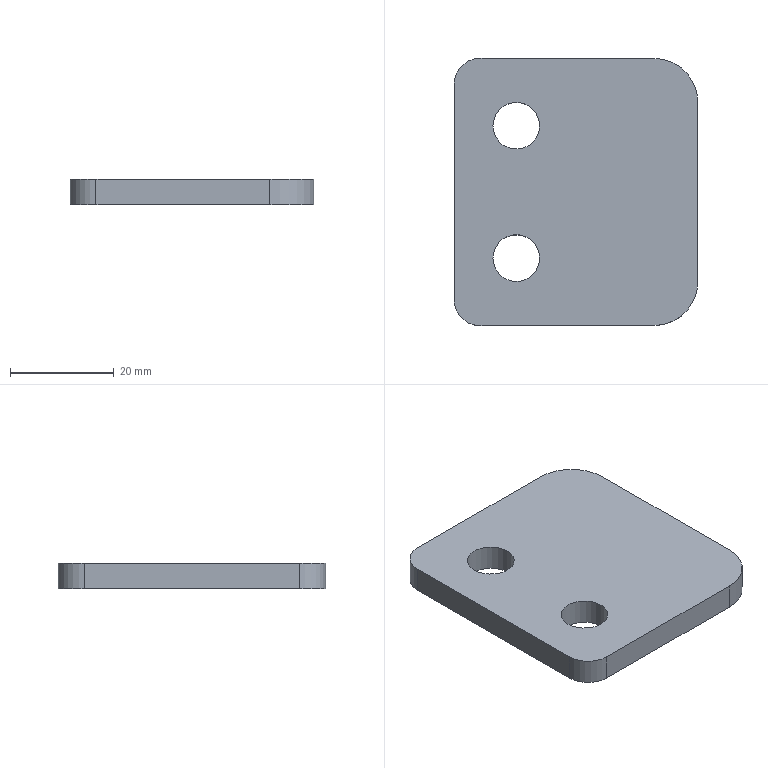Part | STEP file | gslz 2016.10.28-10_id1414_x_t | 1 solid | 12 faces | box 47 x 51.5 x 5 mm | volume 11258 mm3 | cylinder 6 | plane 6 | commonest cylinder face diameters 9 x2 10 x2 17 x2
STEP:
#1=CARTESIAN_POINT('',(0.,0.,0.));
#2=DIRECTION('',(0.,0.,1.));
#3=DIRECTION('',(1.,0.,0.));
#4=AXIS2_PLACEMENT_3D('',#1,#2,#3);
#5=CARTESIAN_POINT('',(-692.25,63.749,15.));
#6=VERTEX_POINT('',#5);
#7=CARTESIAN_POINT('',(-683.75,72.249,15.));
#8=VERTEX_POINT('',#7);
#9=CARTESIAN_POINT('',(-692.25,72.249,15.));
#10=DIRECTION('',(0.,0.,1.));
#11=DIRECTION('',(1.,0.,0.));
#12=AXIS2_PLACEMENT_3D('',#9,#10,#11);
#13=CIRCLE('',#12,8.5);
#14=CARTESIAN_POINT('',(-692.25,72.249,20.));
#15=DIRECTION('',(0.,0.,-1.));
#16=DIRECTION('',(-1.,0.,0.));
#17=AXIS2_PLACEMENT_3D('',#14,#15,#16);
#18=CYLINDRICAL_SURFACE('',#17,8.5);
#19=CARTESIAN_POINT('',(9.425,5.));
#20=DIRECTION('',(-1.,0.));
#21=VECTOR('',#20,1.);
#22=LINE('',#19,#21);
#23=(GEOMETRIC_REPRESENTATION_CONTEXT(2)PARAMETRIC_REPRESENTATION_CONTEXT()REPRESENTATION_CONTEXT('',''));
#24=DEFINITIONAL_REPRESENTATION('',(#22),#23);
#25=PCURVE('',#18,#24);
#26=CARTESIAN_POINT('',(-698.75,87.749,15.));
#27=DIRECTION('',(0.,0.,-1.));
#28=DIRECTION('',(-1.,0.,0.));
#29=AXIS2_PLACEMENT_3D('',#26,#27,#28);
#30=PLANE('',#29);
#31=CARTESIAN_POINT('',(-15.,-15.5));
#32=CARTESIAN_POINT('',(-15.,-0.7776));
#33=CARTESIAN_POINT('',(-2.25,-8.139));
#34=CARTESIAN_POINT('',(10.5,-15.5));
#35=CARTESIAN_POINT('',(-2.25,-22.861));
#36=CARTESIAN_POINT('',(-15.,-30.222));
#37=CARTESIAN_POINT('',(-15.,-15.5));
#38=(BOUNDED_CURVE()B_SPLINE_CURVE(2,(#31,#32,#33,#34,#35,#36,#37),.UNSPECIFIED.,.T.,.F.)B_SPLINE_CURVE_WITH_KNOTS((1,2,2,2,2,1),(-2.094,0.,2.094,4.189,6.283,8.378),.UNSPECIFIED.)CURVE()GEOMETRIC_REPRESENTATION_ITEM()RATIONAL_B_SPLINE_CURVE((1.,0.5,1.,0.5,1.,0.5,1.))REPRESENTATION_ITEM(''));
#39=(GEOMETRIC_REPRESENTATION_CONTEXT(2)PARAMETRIC_REPRESENTATION_CONTEXT()REPRESENTATION_CONTEXT('',''));
#40=DEFINITIONAL_REPRESENTATION('',(#38),#39);
#41=PCURVE('',#30,#40);
#42=SURFACE_CURVE('',#13,(#25,#41),.PCURVE_S1.);
#43=EDGE_CURVE('',#6,#8,#42,.T.);
#44=ORIENTED_EDGE('',*,*,#43,.T.);
#45=CARTESIAN_POINT('',(-683.75,72.249,20.));
#46=VERTEX_POINT('',#45);
#47=CARTESIAN_POINT('',(-683.75,72.249,20.));
#48=DIRECTION('',(0.,0.,-1.));
#49=VECTOR('',#48,1.);
#50=LINE('',#47,#49);
#51=CARTESIAN_POINT('',(3.142,0.));
#52=DIRECTION('',(0.,1.));
#53=VECTOR('',#52,1.);
#54=LINE('',#51,#53);
#55=(GEOMETRIC_REPRESENTATION_CONTEXT(2)PARAMETRIC_REPRESENTATION_CONTEXT()REPRESENTATION_CONTEXT('',''));
#56=DEFINITIONAL_REPRESENTATION('',(#54),#55);
#57=PCURVE('',#18,#56);
#58=CARTESIAN_POINT('',(-683.75,87.749,20.));
#59=DIRECTION('',(-1.,0.,0.));
#60=DIRECTION('',(0.,0.,1.));
#61=AXIS2_PLACEMENT_3D('',#58,#59,#60);
#62=PLANE('',#61);
#63=CARTESIAN_POINT('',(0.,-15.5));
#64=DIRECTION('',(-1.,0.));
#65=VECTOR('',#64,1.);
#66=LINE('',#63,#65);
#67=(GEOMETRIC_REPRESENTATION_CONTEXT(2)PARAMETRIC_REPRESENTATION_CONTEXT()REPRESENTATION_CONTEXT('',''));
#68=DEFINITIONAL_REPRESENTATION('',(#66),#67);
#69=PCURVE('',#62,#68);
#70=SURFACE_CURVE('',#50,(#57,#69),.PCURVE_S1.);
#71=EDGE_CURVE('',#46,#8,#70,.T.);
#72=ORIENTED_EDGE('',*,*,#71,.F.);
#73=CARTESIAN_POINT('',(-692.25,63.749,20.));
#74=VERTEX_POINT('',#73);
#75=CARTESIAN_POINT('',(-692.25,72.249,20.));
#76=DIRECTION('',(0.,0.,1.));
#77=DIRECTION('',(1.,0.,0.));
#78=AXIS2_PLACEMENT_3D('',#75,#76,#77);
#79=CIRCLE('',#78,8.5);
#80=CARTESIAN_POINT('',(9.425,0.));
#81=DIRECTION('',(-1.,0.));
#82=VECTOR('',#81,1.);
#83=LINE('',#80,#82);
#84=(GEOMETRIC_REPRESENTATION_CONTEXT(2)PARAMETRIC_REPRESENTATION_CONTEXT()REPRESENTATION_CONTEXT('',''));
#85=DEFINITIONAL_REPRESENTATION('',(#83),#84);
#86=PCURVE('',#18,#85);
#87=CARTESIAN_POINT('',(-698.75,87.749,20.));
#88=DIRECTION('',(0.,0.,-1.));
#89=DIRECTION('',(-1.,0.,0.));
#90=AXIS2_PLACEMENT_3D('',#87,#88,#89);
#91=PLANE('',#90);
#92=CARTESIAN_POINT('',(-15.,-15.5));
#93=CARTESIAN_POINT('',(-15.,-0.7776));
#94=CARTESIAN_POINT('',(-2.25,-8.139));
#95=CARTESIAN_POINT('',(10.5,-15.5));
#96=CARTESIAN_POINT('',(-2.25,-22.861));
#97=CARTESIAN_POINT('',(-15.,-30.222));
#98=CARTESIAN_POINT('',(-15.,-15.5));
#99=(BOUNDED_CURVE()B_SPLINE_CURVE(2,(#92,#93,#94,#95,#96,#97,#98),.UNSPECIFIED.,.T.,.F.)B_SPLINE_CURVE_WITH_KNOTS((1,2,2,2,2,1),(-2.094,0.,2.094,4.189,6.283,8.378),.UNSPECIFIED.)CURVE()GEOMETRIC_REPRESENTATION_ITEM()RATIONAL_B_SPLINE_CURVE((1.,0.5,1.,0.5,1.,0.5,1.))REPRESENTATION_ITEM(''));
#100=(GEOMETRIC_REPRESENTATION_CONTEXT(2)PARAMETRIC_REPRESENTATION_CONTEXT()REPRESENTATION_CONTEXT('',''));
#101=DEFINITIONAL_REPRESENTATION('',(#99),#100);
#102=PCURVE('',#91,#101);
#103=SURFACE_CURVE('',#79,(#86,#102),.PCURVE_S1.);
#104=EDGE_CURVE('',#74,#46,#103,.T.);
#105=ORIENTED_EDGE('',*,*,#104,.F.);
#106=CARTESIAN_POINT('',(-692.25,63.749,20.));
#107=DIRECTION('',(0.,0.,-1.));
#108=VECTOR('',#107,1.);
#109=LINE('',#106,#108);
#110=CARTESIAN_POINT('',(4.712,0.));
#111=DIRECTION('',(0.,1.));
#112=VECTOR('',#111,1.);
#113=LINE('',#110,#112);
#114=(GEOMETRIC_REPRESENTATION_CONTEXT(2)PARAMETRIC_REPRESENTATION_CONTEXT()REPRESENTATION_CONTEXT('',''));
#115=DEFINITIONAL_REPRESENTATION('',(#113),#114);
#116=PCURVE('',#18,#115);
#117=CARTESIAN_POINT('',(-698.75,63.749,20.));
#118=DIRECTION('',(0.,-1.,0.));
#119=DIRECTION('',(0.,0.,-1.));
#120=AXIS2_PLACEMENT_3D('',#117,#118,#119);
#121=PLANE('',#120);
#122=CARTESIAN_POINT('',(0.,6.5));
#123=DIRECTION('',(1.,0.));
#124=VECTOR('',#123,1.);
#125=LINE('',#122,#124);
#126=(GEOMETRIC_REPRESENTATION_CONTEXT(2)PARAMETRIC_REPRESENTATION_CONTEXT()REPRESENTATION_CONTEXT('',''));
#127=DEFINITIONAL_REPRESENTATION('',(#125),#126);
#128=PCURVE('',#121,#127);
#129=SURFACE_CURVE('',#109,(#116,#128),.PCURVE_S1.);
#130=EDGE_CURVE('',#74,#6,#129,.T.);
#131=ORIENTED_EDGE('',*,*,#130,.T.);
#132=EDGE_LOOP('',(#44,#72,#105,#131));
#133=FACE_BOUND('',#132,.T.);
#134=ADVANCED_FACE('',(#133),#18,.T.);
#135=CARTESIAN_POINT('',(-683.75,106.749,15.));
#136=VERTEX_POINT('',#135);
#137=CARTESIAN_POINT('',(-683.75,87.749,15.));
#138=DIRECTION('',(0.,1.,0.));
#139=VECTOR('',#138,1.);
#140=LINE('',#137,#139);
#141=CARTESIAN_POINT('',(-5.,0.));
#142=DIRECTION('',(0.,1.));
#143=VECTOR('',#142,1.);
#144=LINE('',#141,#143);
#145=(GEOMETRIC_REPRESENTATION_CONTEXT(2)PARAMETRIC_REPRESENTATION_CONTEXT()REPRESENTATION_CONTEXT('',''));
#146=DEFINITIONAL_REPRESENTATION('',(#144),#145);
#147=PCURVE('',#62,#146);
#148=CARTESIAN_POINT('',(-15.,0.));
#149=DIRECTION('',(0.,1.));
#150=VECTOR('',#149,1.);
#151=LINE('',#148,#150);
#152=(GEOMETRIC_REPRESENTATION_CONTEXT(2)PARAMETRIC_REPRESENTATION_CONTEXT()REPRESENTATION_CONTEXT('',''));
#153=DEFINITIONAL_REPRESENTATION('',(#151),#152);
#154=PCURVE('',#30,#153);
#155=SURFACE_CURVE('',#140,(#147,#154),.PCURVE_S1.);
#156=EDGE_CURVE('',#8,#136,#155,.T.);
#157=ORIENTED_EDGE('',*,*,#156,.T.);
#158=CARTESIAN_POINT('',(-683.75,106.749,20.));
#159=VERTEX_POINT('',#158);
#160=CARTESIAN_POINT('',(-683.75,106.749,20.));
#161=DIRECTION('',(0.,0.,-1.));
#162=VECTOR('',#161,1.);
#163=LINE('',#160,#162);
#164=CARTESIAN_POINT('',(0.,19.));
#165=DIRECTION('',(-1.,0.));
#166=VECTOR('',#165,1.);
#167=LINE('',#164,#166);
#168=(GEOMETRIC_REPRESENTATION_CONTEXT(2)PARAMETRIC_REPRESENTATION_CONTEXT()REPRESENTATION_CONTEXT('',''));
#169=DEFINITIONAL_REPRESENTATION('',(#167),#168);
#170=PCURVE('',#62,#169);
#171=CARTESIAN_POINT('',(-692.25,106.749,20.));
#172=DIRECTION('',(0.,0.,-1.));
#173=DIRECTION('',(-1.,0.,0.));
#174=AXIS2_PLACEMENT_3D('',#171,#172,#173);
#175=CYLINDRICAL_SURFACE('',#174,8.5);
#176=CARTESIAN_POINT('',(3.142,0.));
#177=DIRECTION('',(0.,1.));
#178=VECTOR('',#177,1.);
#179=LINE('',#176,#178);
#180=(GEOMETRIC_REPRESENTATION_CONTEXT(2)PARAMETRIC_REPRESENTATION_CONTEXT()REPRESENTATION_CONTEXT('',''));
#181=DEFINITIONAL_REPRESENTATION('',(#179),#180);
#182=PCURVE('',#175,#181);
#183=SURFACE_CURVE('',#163,(#170,#182),.PCURVE_S1.);
#184=EDGE_CURVE('',#159,#136,#183,.T.);
#185=ORIENTED_EDGE('',*,*,#184,.F.);
#186=CARTESIAN_POINT('',(-683.75,87.749,20.));
#187=DIRECTION('',(0.,1.,0.));
#188=VECTOR('',#187,1.);
#189=LINE('',#186,#188);
#190=CARTESIAN_POINT('',(0.,0.));
#191=DIRECTION('',(0.,1.));
#192=VECTOR('',#191,1.);
#193=LINE('',#190,#192);
#194=(GEOMETRIC_REPRESENTATION_CONTEXT(2)PARAMETRIC_REPRESENTATION_CONTEXT()REPRESENTATION_CONTEXT('',''));
#195=DEFINITIONAL_REPRESENTATION('',(#193),#194);
#196=PCURVE('',#62,#195);
#197=CARTESIAN_POINT('',(-15.,0.));
#198=DIRECTION('',(0.,1.));
#199=VECTOR('',#198,1.);
#200=LINE('',#197,#199);
#201=(GEOMETRIC_REPRESENTATION_CONTEXT(2)PARAMETRIC_REPRESENTATION_CONTEXT()REPRESENTATION_CONTEXT('',''));
#202=DEFINITIONAL_REPRESENTATION('',(#200),#201);
#203=PCURVE('',#91,#202);
#204=SURFACE_CURVE('',#189,(#196,#203),.PCURVE_S1.);
#205=EDGE_CURVE('',#46,#159,#204,.T.);
#206=ORIENTED_EDGE('',*,*,#205,.F.);
#207=ORIENTED_EDGE('',*,*,#71,.T.);
#208=EDGE_LOOP('',(#157,#185,#206,#207));
#209=FACE_BOUND('',#208,.T.);
#210=ADVANCED_FACE('',(#209),#62,.F.);
#211=CARTESIAN_POINT('',(-692.25,115.249,15.));
#212=VERTEX_POINT('',#211);
#213=CARTESIAN_POINT('',(-692.25,106.749,15.));
#214=DIRECTION('',(0.,0.,1.));
#215=DIRECTION('',(1.,0.,0.));
#216=AXIS2_PLACEMENT_3D('',#213,#214,#215);
#217=CIRCLE('',#216,8.5);
#218=CARTESIAN_POINT('',(3.142,5.));
#219=DIRECTION('',(-1.,0.));
#220=VECTOR('',#219,1.);
#221=LINE('',#218,#220);
#222=(GEOMETRIC_REPRESENTATION_CONTEXT(2)PARAMETRIC_REPRESENTATION_CONTEXT()REPRESENTATION_CONTEXT('',''));
#223=DEFINITIONAL_REPRESENTATION('',(#221),#222);
#224=PCURVE('',#175,#223);
#225=CARTESIAN_POINT('',(-15.,19.));
#226=CARTESIAN_POINT('',(-15.,33.722));
#227=CARTESIAN_POINT('',(-2.25,26.361));
#228=CARTESIAN_POINT('',(10.5,19.));
#229=CARTESIAN_POINT('',(-2.25,11.639));
#230=CARTESIAN_POINT('',(-15.,4.278));
#231=CARTESIAN_POINT('',(-15.,19.));
#232=(BOUNDED_CURVE()B_SPLINE_CURVE(2,(#225,#226,#227,#228,#229,#230,#231),.UNSPECIFIED.,.T.,.F.)B_SPLINE_CURVE_WITH_KNOTS((1,2,2,2,2,1),(-2.094,0.,2.094,4.189,6.283,8.378),.UNSPECIFIED.)CURVE()GEOMETRIC_REPRESENTATION_ITEM()RATIONAL_B_SPLINE_CURVE((1.,0.5,1.,0.5,1.,0.5,1.))REPRESENTATION_ITEM(''));
#233=(GEOMETRIC_REPRESENTATION_CONTEXT(2)PARAMETRIC_REPRESENTATION_CONTEXT()REPRESENTATION_CONTEXT('',''));
#234=DEFINITIONAL_REPRESENTATION('',(#232),#233);
#235=PCURVE('',#30,#234);
#236=SURFACE_CURVE('',#217,(#224,#235),.PCURVE_S1.);
#237=EDGE_CURVE('',#136,#212,#236,.T.);
#238=ORIENTED_EDGE('',*,*,#237,.T.);
#239=CARTESIAN_POINT('',(-692.25,115.249,20.));
#240=VERTEX_POINT('',#239);
#241=CARTESIAN_POINT('',(-692.25,115.249,20.));
#242=DIRECTION('',(0.,0.,-1.));
#243=VECTOR('',#242,1.);
#244=LINE('',#241,#243);
#245=CARTESIAN_POINT('',(1.571,0.));
#246=DIRECTION('',(0.,1.));
#247=VECTOR('',#246,1.);
#248=LINE('',#245,#247);
#249=(GEOMETRIC_REPRESENTATION_CONTEXT(2)PARAMETRIC_REPRESENTATION_CONTEXT()REPRESENTATION_CONTEXT('',''));
#250=DEFINITIONAL_REPRESENTATION('',(#248),#249);
#251=PCURVE('',#175,#250);
#252=CARTESIAN_POINT('',(-698.75,115.249,20.));
#253=DIRECTION('',(0.,1.,0.));
#254=DIRECTION('',(0.,0.,1.));
#255=AXIS2_PLACEMENT_3D('',#252,#253,#254);
#256=PLANE('',#255);
#257=CARTESIAN_POINT('',(0.,6.5));
#258=DIRECTION('',(-1.,0.));
#259=VECTOR('',#258,1.);
#260=LINE('',#257,#259);
#261=(GEOMETRIC_REPRESENTATION_CONTEXT(2)PARAMETRIC_REPRESENTATION_CONTEXT()REPRESENTATION_CONTEXT('',''));
#262=DEFINITIONAL_REPRESENTATION('',(#260),#261);
#263=PCURVE('',#256,#262);
#264=SURFACE_CURVE('',#244,(#251,#263),.PCURVE_S1.);
#265=EDGE_CURVE('',#240,#212,#264,.T.);
#266=ORIENTED_EDGE('',*,*,#265,.F.);
#267=CARTESIAN_POINT('',(-692.25,106.749,20.));
#268=DIRECTION('',(0.,0.,1.));
#269=DIRECTION('',(1.,0.,0.));
#270=AXIS2_PLACEMENT_3D('',#267,#268,#269);
#271=CIRCLE('',#270,8.5);
#272=CARTESIAN_POINT('',(3.142,0.));
#273=DIRECTION('',(-1.,0.));
#274=VECTOR('',#273,1.);
#275=LINE('',#272,#274);
#276=(GEOMETRIC_REPRESENTATION_CONTEXT(2)PARAMETRIC_REPRESENTATION_CONTEXT()REPRESENTATION_CONTEXT('',''));
#277=DEFINITIONAL_REPRESENTATION('',(#275),#276);
#278=PCURVE('',#175,#277);
#279=CARTESIAN_POINT('',(-15.,19.));
#280=CARTESIAN_POINT('',(-15.,33.722));
#281=CARTESIAN_POINT('',(-2.25,26.361));
#282=CARTESIAN_POINT('',(10.5,19.));
#283=CARTESIAN_POINT('',(-2.25,11.639));
#284=CARTESIAN_POINT('',(-15.,4.278));
#285=CARTESIAN_POINT('',(-15.,19.));
#286=(BOUNDED_CURVE()B_SPLINE_CURVE(2,(#279,#280,#281,#282,#283,#284,#285),.UNSPECIFIED.,.T.,.F.)B_SPLINE_CURVE_WITH_KNOTS((1,2,2,2,2,1),(-2.094,0.,2.094,4.189,6.283,8.378),.UNSPECIFIED.)CURVE()GEOMETRIC_REPRESENTATION_ITEM()RATIONAL_B_SPLINE_CURVE((1.,0.5,1.,0.5,1.,0.5,1.))REPRESENTATION_ITEM(''));
#287=(GEOMETRIC_REPRESENTATION_CONTEXT(2)PARAMETRIC_REPRESENTATION_CONTEXT()REPRESENTATION_CONTEXT('',''));
#288=DEFINITIONAL_REPRESENTATION('',(#286),#287);
#289=PCURVE('',#91,#288);
#290=SURFACE_CURVE('',#271,(#278,#289),.PCURVE_S1.);
#291=EDGE_CURVE('',#159,#240,#290,.T.);
#292=ORIENTED_EDGE('',*,*,#291,.F.);
#293=ORIENTED_EDGE('',*,*,#184,.T.);
#294=EDGE_LOOP('',(#238,#266,#292,#293));
#295=FACE_BOUND('',#294,.T.);
#296=ADVANCED_FACE('',(#295),#175,.T.);
#297=CARTESIAN_POINT('',(-725.75,115.249,15.));
#298=VERTEX_POINT('',#297);
#299=CARTESIAN_POINT('',(-698.75,115.249,15.));
#300=DIRECTION('',(1.,0.,0.));
#301=VECTOR('',#300,1.);
#302=LINE('',#299,#301);
#303=CARTESIAN_POINT('',(-5.,0.));
#304=DIRECTION('',(0.,1.));
#305=VECTOR('',#304,1.);
#306=LINE('',#303,#305);
#307=(GEOMETRIC_REPRESENTATION_CONTEXT(2)PARAMETRIC_REPRESENTATION_CONTEXT()REPRESENTATION_CONTEXT('',''));
#308=DEFINITIONAL_REPRESENTATION('',(#306),#307);
#309=PCURVE('',#256,#308);
#310=CARTESIAN_POINT('',(0.,27.5));
#311=DIRECTION('',(-1.,0.));
#312=VECTOR('',#311,1.);
#313=LINE('',#310,#312);
#314=(GEOMETRIC_REPRESENTATION_CONTEXT(2)PARAMETRIC_REPRESENTATION_CONTEXT()REPRESENTATION_CONTEXT('',''));
#315=DEFINITIONAL_REPRESENTATION('',(#313),#314);
#316=PCURVE('',#30,#315);
#317=SURFACE_CURVE('',#302,(#309,#316),.PCURVE_S1.);
#318=EDGE_CURVE('',#298,#212,#317,.T.);
#319=ORIENTED_EDGE('',*,*,#318,.F.);
#320=CARTESIAN_POINT('',(-725.75,115.249,20.));
#321=VERTEX_POINT('',#320);
#322=CARTESIAN_POINT('',(-725.75,115.249,20.));
#323=DIRECTION('',(0.,0.,-1.));
#324=VECTOR('',#323,1.);
#325=LINE('',#322,#324);
#326=CARTESIAN_POINT('',(0.,-27.));
#327=DIRECTION('',(-1.,0.));
#328=VECTOR('',#327,1.);
#329=LINE('',#326,#328);
#330=(GEOMETRIC_REPRESENTATION_CONTEXT(2)PARAMETRIC_REPRESENTATION_CONTEXT()REPRESENTATION_CONTEXT('',''));
#331=DEFINITIONAL_REPRESENTATION('',(#329),#330);
#332=PCURVE('',#256,#331);
#333=CARTESIAN_POINT('',(-725.75,110.249,20.));
#334=DIRECTION('',(0.,0.,-1.));
#335=DIRECTION('',(-1.,0.,0.));
#336=AXIS2_PLACEMENT_3D('',#333,#334,#335);
#337=CYLINDRICAL_SURFACE('',#336,5.);
#338=CARTESIAN_POINT('',(1.571,0.));
#339=DIRECTION('',(0.,1.));
#340=VECTOR('',#339,1.);
#341=LINE('',#338,#340);
#342=(GEOMETRIC_REPRESENTATION_CONTEXT(2)PARAMETRIC_REPRESENTATION_CONTEXT()REPRESENTATION_CONTEXT('',''));
#343=DEFINITIONAL_REPRESENTATION('',(#341),#342);
#344=PCURVE('',#337,#343);
#345=SURFACE_CURVE('',#325,(#332,#344),.PCURVE_S1.);
#346=EDGE_CURVE('',#321,#298,#345,.T.);
#347=ORIENTED_EDGE('',*,*,#346,.F.);
#348=CARTESIAN_POINT('',(-698.75,115.249,20.));
#349=DIRECTION('',(1.,0.,0.));
#350=VECTOR('',#349,1.);
#351=LINE('',#348,#350);
#352=CARTESIAN_POINT('',(0.,0.));
#353=DIRECTION('',(0.,1.));
#354=VECTOR('',#353,1.);
#355=LINE('',#352,#354);
#356=(GEOMETRIC_REPRESENTATION_CONTEXT(2)PARAMETRIC_REPRESENTATION_CONTEXT()REPRESENTATION_CONTEXT('',''));
#357=DEFINITIONAL_REPRESENTATION('',(#355),#356);
#358=PCURVE('',#256,#357);
#359=CARTESIAN_POINT('',(0.,27.5));
#360=DIRECTION('',(-1.,0.));
#361=VECTOR('',#360,1.);
#362=LINE('',#359,#361);
#363=(GEOMETRIC_REPRESENTATION_CONTEXT(2)PARAMETRIC_REPRESENTATION_CONTEXT()REPRESENTATION_CONTEXT('',''));
#364=DEFINITIONAL_REPRESENTATION('',(#362),#363);
#365=PCURVE('',#91,#364);
#366=SURFACE_CURVE('',#351,(#358,#365),.PCURVE_S1.);
#367=EDGE_CURVE('',#321,#240,#366,.T.);
#368=ORIENTED_EDGE('',*,*,#367,.T.);
#369=ORIENTED_EDGE('',*,*,#265,.T.);
#370=EDGE_LOOP('',(#319,#347,#368,#369));
#371=FACE_BOUND('',#370,.T.);
#372=ADVANCED_FACE('',(#371),#256,.T.);
#373=CARTESIAN_POINT('',(-730.75,110.249,15.));
#374=VERTEX_POINT('',#373);
#375=CARTESIAN_POINT('',(-725.75,110.249,15.));
#376=DIRECTION('',(0.,0.,1.));
#377=DIRECTION('',(1.,0.,0.));
#378=AXIS2_PLACEMENT_3D('',#375,#376,#377);
#379=CIRCLE('',#378,5.);
#380=CARTESIAN_POINT('',(3.142,5.));
#381=DIRECTION('',(-1.,0.));
#382=VECTOR('',#381,1.);
#383=LINE('',#380,#382);
#384=(GEOMETRIC_REPRESENTATION_CONTEXT(2)PARAMETRIC_REPRESENTATION_CONTEXT()REPRESENTATION_CONTEXT('',''));
#385=DEFINITIONAL_REPRESENTATION('',(#383),#384);
#386=PCURVE('',#337,#385);
#387=CARTESIAN_POINT('',(22.,22.5));
#388=CARTESIAN_POINT('',(22.,31.16));
#389=CARTESIAN_POINT('',(29.5,26.83));
#390=CARTESIAN_POINT('',(37.,22.5));
#391=CARTESIAN_POINT('',(29.5,18.17));
#392=CARTESIAN_POINT('',(22.,13.84));
#393=CARTESIAN_POINT('',(22.,22.5));
#394=(BOUNDED_CURVE()B_SPLINE_CURVE(2,(#387,#388,#389,#390,#391,#392,#393),.UNSPECIFIED.,.T.,.F.)B_SPLINE_CURVE_WITH_KNOTS((1,2,2,2,2,1),(-2.094,0.,2.094,4.189,6.283,8.378),.UNSPECIFIED.)CURVE()GEOMETRIC_REPRESENTATION_ITEM()RATIONAL_B_SPLINE_CURVE((1.,0.5,1.,0.5,1.,0.5,1.))REPRESENTATION_ITEM(''));
#395=(GEOMETRIC_REPRESENTATION_CONTEXT(2)PARAMETRIC_REPRESENTATION_CONTEXT()REPRESENTATION_CONTEXT('',''));
#396=DEFINITIONAL_REPRESENTATION('',(#394),#395);
#397=PCURVE('',#30,#396);
#398=SURFACE_CURVE('',#379,(#386,#397),.PCURVE_S1.);
#399=EDGE_CURVE('',#298,#374,#398,.T.);
#400=ORIENTED_EDGE('',*,*,#399,.T.);
#401=CARTESIAN_POINT('',(-730.75,110.249,20.));
#402=VERTEX_POINT('',#401);
#403=CARTESIAN_POINT('',(-730.75,110.249,20.));
#404=DIRECTION('',(0.,0.,-1.));
#405=VECTOR('',#404,1.);
#406=LINE('',#403,#405);
#407=CARTESIAN_POINT('',(0.,0.));
#408=DIRECTION('',(0.,1.));
#409=VECTOR('',#408,1.);
#410=LINE('',#407,#409);
#411=(GEOMETRIC_REPRESENTATION_CONTEXT(2)PARAMETRIC_REPRESENTATION_CONTEXT()REPRESENTATION_CONTEXT('',''));
#412=DEFINITIONAL_REPRESENTATION('',(#410),#411);
#413=PCURVE('',#337,#412);
#414=CARTESIAN_POINT('',(-730.75,87.749,20.));
#415=DIRECTION('',(-1.,0.,0.));
#416=DIRECTION('',(0.,0.,1.));
#417=AXIS2_PLACEMENT_3D('',#414,#415,#416);
#418=PLANE('',#417);
#419=CARTESIAN_POINT('',(0.,22.5));
#420=DIRECTION('',(-1.,0.));
#421=VECTOR('',#420,1.);
#422=LINE('',#419,#421);
#423=(GEOMETRIC_REPRESENTATION_CONTEXT(2)PARAMETRIC_REPRESENTATION_CONTEXT()REPRESENTATION_CONTEXT('',''));
#424=DEFINITIONAL_REPRESENTATION('',(#422),#423);
#425=PCURVE('',#418,#424);
#426=SURFACE_CURVE('',#406,(#413,#425),.PCURVE_S1.);
#427=EDGE_CURVE('',#402,#374,#426,.T.);
#428=ORIENTED_EDGE('',*,*,#427,.F.);
#429=CARTESIAN_POINT('',(-725.75,110.249,20.));
#430=DIRECTION('',(0.,0.,1.));
#431=DIRECTION('',(1.,0.,0.));
#432=AXIS2_PLACEMENT_3D('',#429,#430,#431);
#433=CIRCLE('',#432,5.);
#434=CARTESIAN_POINT('',(3.142,0.));
#435=DIRECTION('',(-1.,0.));
#436=VECTOR('',#435,1.);
#437=LINE('',#434,#436);
#438=(GEOMETRIC_REPRESENTATION_CONTEXT(2)PARAMETRIC_REPRESENTATION_CONTEXT()REPRESENTATION_CONTEXT('',''));
#439=DEFINITIONAL_REPRESENTATION('',(#437),#438);
#440=PCURVE('',#337,#439);
#441=CARTESIAN_POINT('',(22.,22.5));
#442=CARTESIAN_POINT('',(22.,31.16));
#443=CARTESIAN_POINT('',(29.5,26.83));
#444=CARTESIAN_POINT('',(37.,22.5));
#445=CARTESIAN_POINT('',(29.5,18.17));
#446=CARTESIAN_POINT('',(22.,13.84));
#447=CARTESIAN_POINT('',(22.,22.5));
#448=(BOUNDED_CURVE()B_SPLINE_CURVE(2,(#441,#442,#443,#444,#445,#446,#447),.UNSPECIFIED.,.T.,.F.)B_SPLINE_CURVE_WITH_KNOTS((1,2,2,2,2,1),(-2.094,0.,2.094,4.189,6.283,8.378),.UNSPECIFIED.)CURVE()GEOMETRIC_REPRESENTATION_ITEM()RATIONAL_B_SPLINE_CURVE((1.,0.5,1.,0.5,1.,0.5,1.))REPRESENTATION_ITEM(''));
#449=(GEOMETRIC_REPRESENTATION_CONTEXT(2)PARAMETRIC_REPRESENTATION_CONTEXT()REPRESENTATION_CONTEXT('',''));
#450=DEFINITIONAL_REPRESENTATION('',(#448),#449);
#451=PCURVE('',#91,#450);
#452=SURFACE_CURVE('',#433,(#440,#451),.PCURVE_S1.);
#453=EDGE_CURVE('',#321,#402,#452,.T.);
#454=ORIENTED_EDGE('',*,*,#453,.F.);
#455=ORIENTED_EDGE('',*,*,#346,.T.);
#456=EDGE_LOOP('',(#400,#428,#454,#455));
#457=FACE_BOUND('',#456,.T.);
#458=ADVANCED_FACE('',(#457),#337,.T.);
#459=CARTESIAN_POINT('',(-730.75,68.749,15.));
#460=VERTEX_POINT('',#459);
#461=CARTESIAN_POINT('',(-730.75,87.749,15.));
#462=DIRECTION('',(0.,1.,0.));
#463=VECTOR('',#462,1.);
#464=LINE('',#461,#463);
#465=CARTESIAN_POINT('',(-5.,0.));
#466=DIRECTION('',(0.,1.));
#467=VECTOR('',#466,1.);
#468=LINE('',#465,#467);
#469=(GEOMETRIC_REPRESENTATION_CONTEXT(2)PARAMETRIC_REPRESENTATION_CONTEXT()REPRESENTATION_CONTEXT('',''));
#470=DEFINITIONAL_REPRESENTATION('',(#468),#469);
#471=PCURVE('',#418,#470);
#472=CARTESIAN_POINT('',(32.,0.));
#473=DIRECTION('',(0.,1.));
#474=VECTOR('',#473,1.);
#475=LINE('',#472,#474);
#476=(GEOMETRIC_REPRESENTATION_CONTEXT(2)PARAMETRIC_REPRESENTATION_CONTEXT()REPRESENTATION_CONTEXT('',''));
#477=DEFINITIONAL_REPRESENTATION('',(#475),#476);
#478=PCURVE('',#30,#477);
#479=SURFACE_CURVE('',#464,(#471,#478),.PCURVE_S1.);
#480=EDGE_CURVE('',#460,#374,#479,.T.);
#481=ORIENTED_EDGE('',*,*,#480,.F.);
#482=CARTESIAN_POINT('',(-730.75,68.749,20.));
#483=VERTEX_POINT('',#482);
#484=CARTESIAN_POINT('',(-730.75,68.749,20.));
#485=DIRECTION('',(0.,0.,-1.));
#486=VECTOR('',#485,1.);
#487=LINE('',#484,#486);
#488=CARTESIAN_POINT('',(0.,-19.));
#489=DIRECTION('',(-1.,0.));
#490=VECTOR('',#489,1.);
#491=LINE('',#488,#490);
#492=(GEOMETRIC_REPRESENTATION_CONTEXT(2)PARAMETRIC_REPRESENTATION_CONTEXT()REPRESENTATION_CONTEXT('',''));
#493=DEFINITIONAL_REPRESENTATION('',(#491),#492);
#494=PCURVE('',#418,#493);
#495=CARTESIAN_POINT('',(-725.75,68.749,20.));
#496=DIRECTION('',(0.,0.,-1.));
#497=DIRECTION('',(-1.,0.,0.));
#498=AXIS2_PLACEMENT_3D('',#495,#496,#497);
#499=CYLINDRICAL_SURFACE('',#498,5.);
#500=CARTESIAN_POINT('',(6.283,0.));
#501=DIRECTION('',(0.,1.));
#502=VECTOR('',#501,1.);
#503=LINE('',#500,#502);
#504=(GEOMETRIC_REPRESENTATION_CONTEXT(2)PARAMETRIC_REPRESENTATION_CONTEXT()REPRESENTATION_CONTEXT('',''));
#505=DEFINITIONAL_REPRESENTATION('',(#503),#504);
#506=PCURVE('',#499,#505);
#507=SURFACE_CURVE('',#487,(#494,#506),.PCURVE_S1.);
#508=EDGE_CURVE('',#483,#460,#507,.T.);
#509=ORIENTED_EDGE('',*,*,#508,.F.);
#510=CARTESIAN_POINT('',(-730.75,87.749,20.));
#511=DIRECTION('',(0.,1.,0.));
#512=VECTOR('',#511,1.);
#513=LINE('',#510,#512);
#514=CARTESIAN_POINT('',(0.,0.));
#515=DIRECTION('',(0.,1.));
#516=VECTOR('',#515,1.);
#517=LINE('',#514,#516);
#518=(GEOMETRIC_REPRESENTATION_CONTEXT(2)PARAMETRIC_REPRESENTATION_CONTEXT()REPRESENTATION_CONTEXT('',''));
#519=DEFINITIONAL_REPRESENTATION('',(#517),#518);
#520=PCURVE('',#418,#519);
#521=CARTESIAN_POINT('',(32.,0.));
#522=DIRECTION('',(0.,1.));
#523=VECTOR('',#522,1.);
#524=LINE('',#521,#523);
#525=(GEOMETRIC_REPRESENTATION_CONTEXT(2)PARAMETRIC_REPRESENTATION_CONTEXT()REPRESENTATION_CONTEXT('',''));
#526=DEFINITIONAL_REPRESENTATION('',(#524),#525);
#527=PCURVE('',#91,#526);
#528=SURFACE_CURVE('',#513,(#520,#527),.PCURVE_S1.);
#529=EDGE_CURVE('',#483,#402,#528,.T.);
#530=ORIENTED_EDGE('',*,*,#529,.T.);
#531=ORIENTED_EDGE('',*,*,#427,.T.);
#532=EDGE_LOOP('',(#481,#509,#530,#531));
#533=FACE_BOUND('',#532,.T.);
#534=ADVANCED_FACE('',(#533),#418,.T.);
#535=CARTESIAN_POINT('',(-725.75,63.749,15.));
#536=VERTEX_POINT('',#535);
#537=CARTESIAN_POINT('',(-725.75,68.749,15.));
#538=DIRECTION('',(0.,0.,1.));
#539=DIRECTION('',(1.,0.,0.));
#540=AXIS2_PLACEMENT_3D('',#537,#538,#539);
#541=CIRCLE('',#540,5.);
#542=CARTESIAN_POINT('',(9.425,5.));
#543=DIRECTION('',(-1.,0.));
#544=VECTOR('',#543,1.);
#545=LINE('',#542,#544);
#546=(GEOMETRIC_REPRESENTATION_CONTEXT(2)PARAMETRIC_REPRESENTATION_CONTEXT()REPRESENTATION_CONTEXT('',''));
#547=DEFINITIONAL_REPRESENTATION('',(#545),#546);
#548=PCURVE('',#499,#547);
#549=CARTESIAN_POINT('',(22.,-19.));
#550=CARTESIAN_POINT('',(22.,-10.34));
#551=CARTESIAN_POINT('',(29.5,-14.67));
#552=CARTESIAN_POINT('',(37.,-19.));
#553=CARTESIAN_POINT('',(29.5,-23.33));
#554=CARTESIAN_POINT('',(22.,-27.66));
#555=CARTESIAN_POINT('',(22.,-19.));
#556=(BOUNDED_CURVE()B_SPLINE_CURVE(2,(#549,#550,#551,#552,#553,#554,#555),.UNSPECIFIED.,.T.,.F.)B_SPLINE_CURVE_WITH_KNOTS((1,2,2,2,2,1),(-2.094,0.,2.094,4.189,6.283,8.378),.UNSPECIFIED.)CURVE()GEOMETRIC_REPRESENTATION_ITEM()RATIONAL_B_SPLINE_CURVE((1.,0.5,1.,0.5,1.,0.5,1.))REPRESENTATION_ITEM(''));
#557=(GEOMETRIC_REPRESENTATION_CONTEXT(2)PARAMETRIC_REPRESENTATION_CONTEXT()REPRESENTATION_CONTEXT('',''));
#558=DEFINITIONAL_REPRESENTATION('',(#556),#557);
#559=PCURVE('',#30,#558);
#560=SURFACE_CURVE('',#541,(#548,#559),.PCURVE_S1.);
#561=EDGE_CURVE('',#460,#536,#560,.T.);
#562=ORIENTED_EDGE('',*,*,#561,.T.);
#563=CARTESIAN_POINT('',(-725.75,63.749,20.));
#564=VERTEX_POINT('',#563);
#565=CARTESIAN_POINT('',(-725.75,63.749,20.));
#566=DIRECTION('',(0.,0.,-1.));
#567=VECTOR('',#566,1.);
#568=LINE('',#565,#567);
#569=CARTESIAN_POINT('',(4.712,0.));
#570=DIRECTION('',(0.,1.));
#571=VECTOR('',#570,1.);
#572=LINE('',#569,#571);
#573=(GEOMETRIC_REPRESENTATION_CONTEXT(2)PARAMETRIC_REPRESENTATION_CONTEXT()REPRESENTATION_CONTEXT('',''));
#574=DEFINITIONAL_REPRESENTATION('',(#572),#573);
#575=PCURVE('',#499,#574);
#576=CARTESIAN_POINT('',(0.,-27.));
#577=DIRECTION('',(1.,0.));
#578=VECTOR('',#577,1.);
#579=LINE('',#576,#578);
#580=(GEOMETRIC_REPRESENTATION_CONTEXT(2)PARAMETRIC_REPRESENTATION_CONTEXT()REPRESENTATION_CONTEXT('',''));
#581=DEFINITIONAL_REPRESENTATION('',(#579),#580);
#582=PCURVE('',#121,#581);
#583=SURFACE_CURVE('',#568,(#575,#582),.PCURVE_S1.);
#584=EDGE_CURVE('',#564,#536,#583,.T.);
#585=ORIENTED_EDGE('',*,*,#584,.F.);
#586=CARTESIAN_POINT('',(-725.75,68.749,20.));
#587=DIRECTION('',(0.,0.,1.));
#588=DIRECTION('',(1.,0.,0.));
#589=AXIS2_PLACEMENT_3D('',#586,#587,#588);
#590=CIRCLE('',#589,5.);
#591=CARTESIAN_POINT('',(9.425,0.));
#592=DIRECTION('',(-1.,0.));
#593=VECTOR('',#592,1.);
#594=LINE('',#591,#593);
#595=(GEOMETRIC_REPRESENTATION_CONTEXT(2)PARAMETRIC_REPRESENTATION_CONTEXT()REPRESENTATION_CONTEXT('',''));
#596=DEFINITIONAL_REPRESENTATION('',(#594),#595);
#597=PCURVE('',#499,#596);
#598=CARTESIAN_POINT('',(22.,-19.));
#599=CARTESIAN_POINT('',(22.,-10.34));
#600=CARTESIAN_POINT('',(29.5,-14.67));
#601=CARTESIAN_POINT('',(37.,-19.));
#602=CARTESIAN_POINT('',(29.5,-23.33));
#603=CARTESIAN_POINT('',(22.,-27.66));
#604=CARTESIAN_POINT('',(22.,-19.));
#605=(BOUNDED_CURVE()B_SPLINE_CURVE(2,(#598,#599,#600,#601,#602,#603,#604),.UNSPECIFIED.,.T.,.F.)B_SPLINE_CURVE_WITH_KNOTS((1,2,2,2,2,1),(-2.094,0.,2.094,4.189,6.283,8.378),.UNSPECIFIED.)CURVE()GEOMETRIC_REPRESENTATION_ITEM()RATIONAL_B_SPLINE_CURVE((1.,0.5,1.,0.5,1.,0.5,1.))REPRESENTATION_ITEM(''));
#606=(GEOMETRIC_REPRESENTATION_CONTEXT(2)PARAMETRIC_REPRESENTATION_CONTEXT()REPRESENTATION_CONTEXT('',''));
#607=DEFINITIONAL_REPRESENTATION('',(#605),#606);
#608=PCURVE('',#91,#607);
#609=SURFACE_CURVE('',#590,(#597,#608),.PCURVE_S1.);
#610=EDGE_CURVE('',#483,#564,#609,.T.);
#611=ORIENTED_EDGE('',*,*,#610,.F.);
#612=ORIENTED_EDGE('',*,*,#508,.T.);
#613=EDGE_LOOP('',(#562,#585,#611,#612));
#614=FACE_BOUND('',#613,.T.);
#615=ADVANCED_FACE('',(#614),#499,.T.);
#616=CARTESIAN_POINT('',(-723.25,102.249,20.));
#617=VERTEX_POINT('',#616);
#618=CARTESIAN_POINT('',(-718.75,102.249,20.));
#619=DIRECTION('',(0.,0.,-1.));
#620=DIRECTION('',(-1.,0.,0.));
#621=AXIS2_PLACEMENT_3D('',#618,#619,#620);
#622=CIRCLE('',#621,4.5);
#623=CARTESIAN_POINT('',(-718.75,102.249,20.));
#624=DIRECTION('',(0.,0.,-1.));
#625=DIRECTION('',(-1.,0.,0.));
#626=AXIS2_PLACEMENT_3D('',#623,#624,#625);
#627=CYLINDRICAL_SURFACE('',#626,4.5);
#628=CARTESIAN_POINT('',(0.,0.));
#629=DIRECTION('',(1.,0.));
#630=VECTOR('',#629,1.);
#631=LINE('',#628,#630);
#632=(GEOMETRIC_REPRESENTATION_CONTEXT(2)PARAMETRIC_REPRESENTATION_CONTEXT()REPRESENTATION_CONTEXT('',''));
#633=DEFINITIONAL_REPRESENTATION('',(#631),#632);
#634=PCURVE('',#627,#633);
#635=CARTESIAN_POINT('',(20.,14.5));
#636=DIRECTION('',(1.,0.));
#637=AXIS2_PLACEMENT_2D('',#635,#636);
#638=CIRCLE('',#637,4.5);
#639=(GEOMETRIC_REPRESENTATION_CONTEXT(2)PARAMETRIC_REPRESENTATION_CONTEXT()REPRESENTATION_CONTEXT('',''));
#640=DEFINITIONAL_REPRESENTATION('',(#638),#639);
#641=PCURVE('',#91,#640);
#642=SURFACE_CURVE('',#622,(#634,#641),.PCURVE_S1.);
#643=EDGE_CURVE('',#617,#617,#642,.T.);
#644=ORIENTED_EDGE('',*,*,#643,.T.);
#645=CARTESIAN_POINT('',(-723.25,102.249,15.));
#646=VERTEX_POINT('',#645);
#647=CARTESIAN_POINT('',(-723.25,102.249,20.));
#648=CARTESIAN_POINT('',(-723.25,102.249,15.));
#649=B_SPLINE_CURVE_WITH_KNOTS('',1,(#647,#648),.UNSPECIFIED.,.F.,.F.,(2,2),(0.,5.),.PIECEWISE_BEZIER_KNOTS.);
#650=CARTESIAN_POINT('',(6.283,0.));
#651=DIRECTION('',(0.,1.));
#652=VECTOR('',#651,1.);
#653=LINE('',#650,#652);
#654=(GEOMETRIC_REPRESENTATION_CONTEXT(2)PARAMETRIC_REPRESENTATION_CONTEXT()REPRESENTATION_CONTEXT('',''));
#655=DEFINITIONAL_REPRESENTATION('',(#653),#654);
#656=PCURVE('',#627,#655);
#657=CARTESIAN_POINT('',(0.,0.));
#658=DIRECTION('',(0.,1.));
#659=VECTOR('',#658,1.);
#660=LINE('',#657,#659);
#661=(GEOMETRIC_REPRESENTATION_CONTEXT(2)PARAMETRIC_REPRESENTATION_CONTEXT()REPRESENTATION_CONTEXT('',''));
#662=DEFINITIONAL_REPRESENTATION('',(#660),#661);
#663=PCURVE('',#627,#662);
#664=SEAM_CURVE('',#649,(#656,#663),.PCURVE_S1.);
#665=EDGE_CURVE('',#617,#646,#664,.T.);
#666=ORIENTED_EDGE('',*,*,#665,.T.);
#667=CARTESIAN_POINT('',(-718.75,102.249,15.));
#668=DIRECTION('',(0.,0.,-1.));
#669=DIRECTION('',(-1.,0.,0.));
#670=AXIS2_PLACEMENT_3D('',#667,#668,#669);
#671=CIRCLE('',#670,4.5);
#672=CARTESIAN_POINT('',(0.,5.));
#673=DIRECTION('',(1.,0.));
#674=VECTOR('',#673,1.);
#675=LINE('',#672,#674);
#676=(GEOMETRIC_REPRESENTATION_CONTEXT(2)PARAMETRIC_REPRESENTATION_CONTEXT()REPRESENTATION_CONTEXT('',''));
#677=DEFINITIONAL_REPRESENTATION('',(#675),#676);
#678=PCURVE('',#627,#677);
#679=CARTESIAN_POINT('',(20.,14.5));
#680=DIRECTION('',(1.,0.));
#681=AXIS2_PLACEMENT_2D('',#679,#680);
#682=CIRCLE('',#681,4.5);
#683=(GEOMETRIC_REPRESENTATION_CONTEXT(2)PARAMETRIC_REPRESENTATION_CONTEXT()REPRESENTATION_CONTEXT('',''));
#684=DEFINITIONAL_REPRESENTATION('',(#682),#683);
#685=PCURVE('',#30,#684);
#686=SURFACE_CURVE('',#671,(#678,#685),.PCURVE_S1.);
#687=EDGE_CURVE('',#646,#646,#686,.T.);
#688=ORIENTED_EDGE('',*,*,#687,.F.);
#689=ORIENTED_EDGE('',*,*,#665,.F.);
#690=EDGE_LOOP('',(#644,#666,#688,#689));
#691=FACE_BOUND('',#690,.F.);
#692=ADVANCED_FACE('',(#691),#627,.F.);
#693=CARTESIAN_POINT('',(-723.25,76.749,20.));
#694=VERTEX_POINT('',#693);
#695=CARTESIAN_POINT('',(-718.75,76.749,20.));
#696=DIRECTION('',(0.,0.,-1.));
#697=DIRECTION('',(-1.,0.,0.));
#698=AXIS2_PLACEMENT_3D('',#695,#696,#697);
#699=CIRCLE('',#698,4.5);
#700=CARTESIAN_POINT('',(-718.75,76.749,20.));
#701=DIRECTION('',(0.,0.,-1.));
#702=DIRECTION('',(-1.,0.,0.));
#703=AXIS2_PLACEMENT_3D('',#700,#701,#702);
#704=CYLINDRICAL_SURFACE('',#703,4.5);
#705=CARTESIAN_POINT('',(0.,0.));
#706=DIRECTION('',(1.,0.));
#707=VECTOR('',#706,1.);
#708=LINE('',#705,#707);
#709=(GEOMETRIC_REPRESENTATION_CONTEXT(2)PARAMETRIC_REPRESENTATION_CONTEXT()REPRESENTATION_CONTEXT('',''));
#710=DEFINITIONAL_REPRESENTATION('',(#708),#709);
#711=PCURVE('',#704,#710);
#712=CARTESIAN_POINT('',(20.,-11.));
#713=DIRECTION('',(1.,0.));
#714=AXIS2_PLACEMENT_2D('',#712,#713);
#715=CIRCLE('',#714,4.5);
#716=(GEOMETRIC_REPRESENTATION_CONTEXT(2)PARAMETRIC_REPRESENTATION_CONTEXT()REPRESENTATION_CONTEXT('',''));
#717=DEFINITIONAL_REPRESENTATION('',(#715),#716);
#718=PCURVE('',#91,#717);
#719=SURFACE_CURVE('',#699,(#711,#718),.PCURVE_S1.);
#720=EDGE_CURVE('',#694,#694,#719,.T.);
#721=ORIENTED_EDGE('',*,*,#720,.T.);
#722=CARTESIAN_POINT('',(-723.25,76.749,15.));
#723=VERTEX_POINT('',#722);
#724=CARTESIAN_POINT('',(-723.25,76.749,20.));
#725=CARTESIAN_POINT('',(-723.25,76.749,15.));
#726=B_SPLINE_CURVE_WITH_KNOTS('',1,(#724,#725),.UNSPECIFIED.,.F.,.F.,(2,2),(0.,5.),.PIECEWISE_BEZIER_KNOTS.);
#727=CARTESIAN_POINT('',(6.283,0.));
#728=DIRECTION('',(0.,1.));
#729=VECTOR('',#728,1.);
#730=LINE('',#727,#729);
#731=(GEOMETRIC_REPRESENTATION_CONTEXT(2)PARAMETRIC_REPRESENTATION_CONTEXT()REPRESENTATION_CONTEXT('',''));
#732=DEFINITIONAL_REPRESENTATION('',(#730),#731);
#733=PCURVE('',#704,#732);
#734=CARTESIAN_POINT('',(0.,0.));
#735=DIRECTION('',(0.,1.));
#736=VECTOR('',#735,1.);
#737=LINE('',#734,#736);
#738=(GEOMETRIC_REPRESENTATION_CONTEXT(2)PARAMETRIC_REPRESENTATION_CONTEXT()REPRESENTATION_CONTEXT('',''));
#739=DEFINITIONAL_REPRESENTATION('',(#737),#738);
#740=PCURVE('',#704,#739);
#741=SEAM_CURVE('',#726,(#733,#740),.PCURVE_S1.);
#742=EDGE_CURVE('',#694,#723,#741,.T.);
#743=ORIENTED_EDGE('',*,*,#742,.T.);
#744=CARTESIAN_POINT('',(-718.75,76.749,15.));
#745=DIRECTION('',(0.,0.,-1.));
#746=DIRECTION('',(-1.,0.,0.));
#747=AXIS2_PLACEMENT_3D('',#744,#745,#746);
#748=CIRCLE('',#747,4.5);
#749=CARTESIAN_POINT('',(0.,5.));
#750=DIRECTION('',(1.,0.));
#751=VECTOR('',#750,1.);
#752=LINE('',#749,#751);
#753=(GEOMETRIC_REPRESENTATION_CONTEXT(2)PARAMETRIC_REPRESENTATION_CONTEXT()REPRESENTATION_CONTEXT('',''));
#754=DEFINITIONAL_REPRESENTATION('',(#752),#753);
#755=PCURVE('',#704,#754);
#756=CARTESIAN_POINT('',(20.,-11.));
#757=DIRECTION('',(1.,0.));
#758=AXIS2_PLACEMENT_2D('',#756,#757);
#759=CIRCLE('',#758,4.5);
#760=(GEOMETRIC_REPRESENTATION_CONTEXT(2)PARAMETRIC_REPRESENTATION_CONTEXT()REPRESENTATION_CONTEXT('',''));
#761=DEFINITIONAL_REPRESENTATION('',(#759),#760);
#762=PCURVE('',#30,#761);
#763=SURFACE_CURVE('',#748,(#755,#762),.PCURVE_S1.);
#764=EDGE_CURVE('',#723,#723,#763,.T.);
#765=ORIENTED_EDGE('',*,*,#764,.F.);
#766=ORIENTED_EDGE('',*,*,#742,.F.);
#767=EDGE_LOOP('',(#721,#743,#765,#766));
#768=FACE_BOUND('',#767,.F.);
#769=ADVANCED_FACE('',(#768),#704,.F.);
#770=CARTESIAN_POINT('',(-698.75,63.749,15.));
#771=DIRECTION('',(-1.,0.,0.));
#772=VECTOR('',#771,1.);
#773=LINE('',#770,#772);
#774=CARTESIAN_POINT('',(5.,0.));
#775=DIRECTION('',(0.,-1.));
#776=VECTOR('',#775,1.);
#777=LINE('',#774,#776);
#778=(GEOMETRIC_REPRESENTATION_CONTEXT(2)PARAMETRIC_REPRESENTATION_CONTEXT()REPRESENTATION_CONTEXT('',''));
#779=DEFINITIONAL_REPRESENTATION('',(#777),#778);
#780=PCURVE('',#121,#779);
#781=CARTESIAN_POINT('',(0.,-24.));
#782=DIRECTION('',(1.,0.));
#783=VECTOR('',#782,1.);
#784=LINE('',#781,#783);
#785=(GEOMETRIC_REPRESENTATION_CONTEXT(2)PARAMETRIC_REPRESENTATION_CONTEXT()REPRESENTATION_CONTEXT('',''));
#786=DEFINITIONAL_REPRESENTATION('',(#784),#785);
#787=PCURVE('',#30,#786);
#788=SURFACE_CURVE('',#773,(#780,#787),.PCURVE_S1.);
#789=EDGE_CURVE('',#6,#536,#788,.T.);
#790=ORIENTED_EDGE('',*,*,#789,.F.);
#791=ORIENTED_EDGE('',*,*,#130,.F.);
#792=CARTESIAN_POINT('',(-698.75,63.749,20.));
#793=DIRECTION('',(-1.,0.,0.));
#794=VECTOR('',#793,1.);
#795=LINE('',#792,#794);
#796=CARTESIAN_POINT('',(0.,0.));
#797=DIRECTION('',(0.,-1.));
#798=VECTOR('',#797,1.);
#799=LINE('',#796,#798);
#800=(GEOMETRIC_REPRESENTATION_CONTEXT(2)PARAMETRIC_REPRESENTATION_CONTEXT()REPRESENTATION_CONTEXT('',''));
#801=DEFINITIONAL_REPRESENTATION('',(#799),#800);
#802=PCURVE('',#121,#801);
#803=CARTESIAN_POINT('',(0.,-24.));
#804=DIRECTION('',(1.,0.));
#805=VECTOR('',#804,1.);
#806=LINE('',#803,#805);
#807=(GEOMETRIC_REPRESENTATION_CONTEXT(2)PARAMETRIC_REPRESENTATION_CONTEXT()REPRESENTATION_CONTEXT('',''));
#808=DEFINITIONAL_REPRESENTATION('',(#806),#807);
#809=PCURVE('',#91,#808);
#810=SURFACE_CURVE('',#795,(#802,#809),.PCURVE_S1.);
#811=EDGE_CURVE('',#74,#564,#810,.T.);
#812=ORIENTED_EDGE('',*,*,#811,.T.);
#813=ORIENTED_EDGE('',*,*,#584,.T.);
#814=EDGE_LOOP('',(#790,#791,#812,#813));
#815=FACE_BOUND('',#814,.T.);
#816=ADVANCED_FACE('',(#815),#121,.T.);
#817=ORIENTED_EDGE('',*,*,#104,.T.);
#818=ORIENTED_EDGE('',*,*,#205,.T.);
#819=ORIENTED_EDGE('',*,*,#291,.T.);
#820=ORIENTED_EDGE('',*,*,#367,.F.);
#821=ORIENTED_EDGE('',*,*,#453,.T.);
#822=ORIENTED_EDGE('',*,*,#529,.F.);
#823=ORIENTED_EDGE('',*,*,#610,.T.);
#824=ORIENTED_EDGE('',*,*,#811,.F.);
#825=EDGE_LOOP('',(#817,#818,#819,#820,#821,#822,#823,#824));
#826=FACE_BOUND('',#825,.T.);
#827=ORIENTED_EDGE('',*,*,#720,.T.);
#828=EDGE_LOOP('',(#827));
#829=FACE_BOUND('',#828,.T.);
#830=ORIENTED_EDGE('',*,*,#643,.T.);
#831=EDGE_LOOP('',(#830));
#832=FACE_BOUND('',#831,.T.);
#833=ADVANCED_FACE('',(#826,#829,#832),#91,.F.);
#834=ORIENTED_EDGE('',*,*,#43,.F.);
#835=ORIENTED_EDGE('',*,*,#789,.T.);
#836=ORIENTED_EDGE('',*,*,#561,.F.);
#837=ORIENTED_EDGE('',*,*,#480,.T.);
#838=ORIENTED_EDGE('',*,*,#399,.F.);
#839=ORIENTED_EDGE('',*,*,#318,.T.);
#840=ORIENTED_EDGE('',*,*,#237,.F.);
#841=ORIENTED_EDGE('',*,*,#156,.F.);
#842=EDGE_LOOP('',(#834,#835,#836,#837,#838,#839,#840,#841));
#843=FACE_BOUND('',#842,.T.);
#844=ORIENTED_EDGE('',*,*,#764,.F.);
#845=EDGE_LOOP('',(#844));
#846=FACE_BOUND('',#845,.T.);
#847=ORIENTED_EDGE('',*,*,#687,.F.);
#848=EDGE_LOOP('',(#847));
#849=FACE_BOUND('',#848,.T.);
#850=ADVANCED_FACE('',(#843,#846,#849),#30,.T.);
#851=CLOSED_SHELL('',(#134,#210,#296,#372,#458,#534,#615,#692,#769,#816,#833,#850));
#852=MANIFOLD_SOLID_BREP('',#851);
#853=(LENGTH_UNIT()NAMED_UNIT(*)SI_UNIT(.MILLI.,.METRE.));
#854=UNCERTAINTY_MEASURE_WITH_UNIT(LENGTH_MEASURE(0.000002),#853,'','');
#855=(NAMED_UNIT(*)PLANE_ANGLE_UNIT()SI_UNIT($,.RADIAN.));
#856=(NAMED_UNIT(*)SI_UNIT($,.STERADIAN.)SOLID_ANGLE_UNIT());
#857=(GEOMETRIC_REPRESENTATION_CONTEXT(3)GLOBAL_UNCERTAINTY_ASSIGNED_CONTEXT((#854))GLOBAL_UNIT_ASSIGNED_CONTEXT((#853,#855,#856))REPRESENTATION_CONTEXT('',''));
#858=ADVANCED_BREP_SHAPE_REPRESENTATION('',(#4,#852),#857);